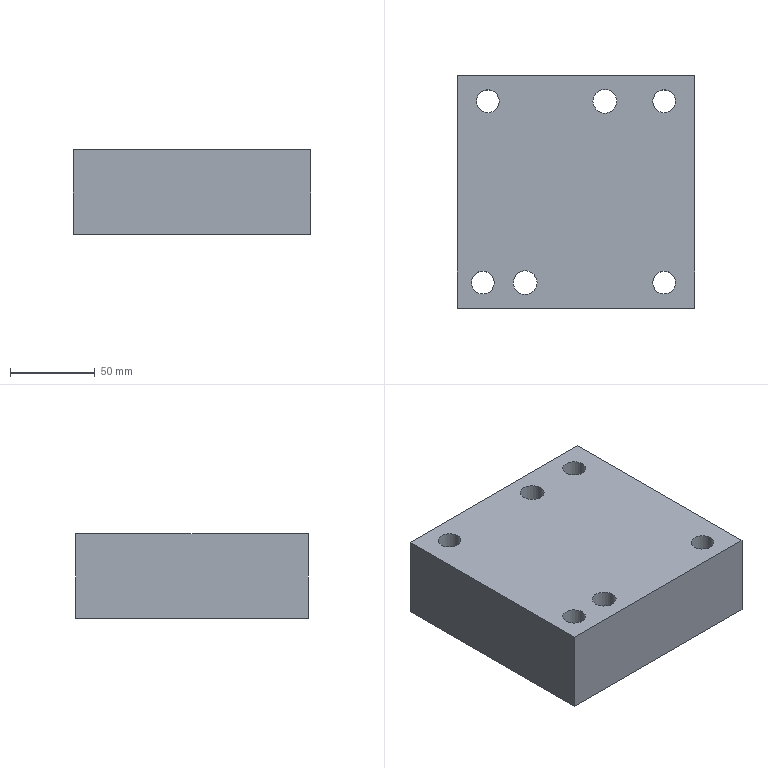Part | STEP file | lll_id3158_x_t | 1 solid | 16 faces | box 140 x 137 x 50 mm | volume 911433 mm3 | cylinder 8 | plane 6 | cone 2 | commonest cylinder face diameters 13.509 x4 8.506 x2 14 x2
STEP:
#1=CARTESIAN_POINT('',(525.125,-377.25,142.5));
#2=VERTEX_POINT('',#1);
#3=CARTESIAN_POINT('',(518.37,-377.25,142.5));
#4=DIRECTION('',(0.,0.,1.));
#5=DIRECTION('',(1.,0.,0.));
#6=AXIS2_PLACEMENT_3D('',#3,#4,#5);
#7=CIRCLE('',#6,6.755);
#8=EDGE_CURVE('',#2,#2,#7,.T.);
#9=ORIENTED_EDGE('',*,*,#8,.F.);
#10=EDGE_LOOP('',(#9));
#11=FACE_BOUND('',#10,.T.);
#12=CARTESIAN_POINT('',(490.371,-270.25,142.5));
#13=VERTEX_POINT('',#12);
#14=CARTESIAN_POINT('',(483.37,-270.25,142.5));
#15=DIRECTION('',(0.,0.,-1.));
#16=DIRECTION('',(1.,0.,0.));
#17=AXIS2_PLACEMENT_3D('',#14,#15,#16);
#18=CIRCLE('',#17,7.);
#19=EDGE_CURVE('',#13,#13,#18,.T.);
#20=ORIENTED_EDGE('',*,*,#19,.T.);
#21=EDGE_LOOP('',(#20));
#22=FACE_BOUND('',#21,.T.);
#23=CARTESIAN_POINT('',(421.125,-270.25,142.5));
#24=VERTEX_POINT('',#23);
#25=CARTESIAN_POINT('',(414.37,-270.25,142.5));
#26=DIRECTION('',(0.,0.,1.));
#27=DIRECTION('',(1.,0.,0.));
#28=AXIS2_PLACEMENT_3D('',#25,#26,#27);
#29=CIRCLE('',#28,6.755);
#30=EDGE_CURVE('',#24,#24,#29,.T.);
#31=ORIENTED_EDGE('',*,*,#30,.F.);
#32=EDGE_LOOP('',(#31));
#33=FACE_BOUND('',#32,.T.);
#34=CARTESIAN_POINT('',(443.371,-377.25,142.5));
#35=VERTEX_POINT('',#34);
#36=CARTESIAN_POINT('',(436.37,-377.25,142.5));
#37=DIRECTION('',(0.,0.,-1.));
#38=DIRECTION('',(1.,0.,0.));
#39=AXIS2_PLACEMENT_3D('',#36,#37,#38);
#40=CIRCLE('',#39,7.);
#41=EDGE_CURVE('',#35,#35,#40,.T.);
#42=ORIENTED_EDGE('',*,*,#41,.T.);
#43=EDGE_LOOP('',(#42));
#44=FACE_BOUND('',#43,.T.);
#45=CARTESIAN_POINT('',(536.37,-255.25,142.5));
#46=VERTEX_POINT('',#45);
#47=CARTESIAN_POINT('',(536.37,-392.25,142.5));
#48=VERTEX_POINT('',#47);
#49=CARTESIAN_POINT('',(536.37,-325.25,142.5));
#50=DIRECTION('',(0.,-1.,0.));
#51=VECTOR('',#50,1.);
#52=LINE('',#49,#51);
#53=EDGE_CURVE('',#46,#48,#52,.T.);
#54=ORIENTED_EDGE('',*,*,#53,.F.);
#55=CARTESIAN_POINT('',(396.37,-255.25,142.5));
#56=VERTEX_POINT('',#55);
#57=CARTESIAN_POINT('',(466.37,-255.25,142.5));
#58=DIRECTION('',(1.,0.,0.));
#59=VECTOR('',#58,1.);
#60=LINE('',#57,#59);
#61=EDGE_CURVE('',#56,#46,#60,.T.);
#62=ORIENTED_EDGE('',*,*,#61,.F.);
#63=CARTESIAN_POINT('',(396.37,-392.25,142.5));
#64=VERTEX_POINT('',#63);
#65=CARTESIAN_POINT('',(396.37,-325.25,142.5));
#66=DIRECTION('',(0.,1.,0.));
#67=VECTOR('',#66,1.);
#68=LINE('',#65,#67);
#69=EDGE_CURVE('',#64,#56,#68,.T.);
#70=ORIENTED_EDGE('',*,*,#69,.F.);
#71=CARTESIAN_POINT('',(466.37,-392.25,142.5));
#72=DIRECTION('',(-1.,0.,0.));
#73=VECTOR('',#72,1.);
#74=LINE('',#71,#73);
#75=EDGE_CURVE('',#48,#64,#74,.T.);
#76=ORIENTED_EDGE('',*,*,#75,.F.);
#77=EDGE_LOOP('',(#54,#62,#70,#76));
#78=FACE_BOUND('',#77,.T.);
#79=CARTESIAN_POINT('',(418.125,-377.25,142.5));
#80=VERTEX_POINT('',#79);
#81=CARTESIAN_POINT('',(411.37,-377.25,142.5));
#82=DIRECTION('',(0.,0.,-1.));
#83=DIRECTION('',(1.,0.,0.));
#84=AXIS2_PLACEMENT_3D('',#81,#82,#83);
#85=CIRCLE('',#84,6.755);
#86=EDGE_CURVE('',#80,#80,#85,.T.);
#87=ORIENTED_EDGE('',*,*,#86,.T.);
#88=EDGE_LOOP('',(#87));
#89=FACE_BOUND('',#88,.T.);
#90=CARTESIAN_POINT('',(525.125,-270.25,142.5));
#91=VERTEX_POINT('',#90);
#92=CARTESIAN_POINT('',(518.37,-270.25,142.5));
#93=DIRECTION('',(0.,0.,-1.));
#94=DIRECTION('',(1.,0.,0.));
#95=AXIS2_PLACEMENT_3D('',#92,#93,#94);
#96=CIRCLE('',#95,6.755);
#97=EDGE_CURVE('',#91,#91,#96,.T.);
#98=ORIENTED_EDGE('',*,*,#97,.T.);
#99=EDGE_LOOP('',(#98));
#100=FACE_BOUND('',#99,.T.);
#101=CARTESIAN_POINT('',(42.419,-273.704,142.5));
#102=DIRECTION('',(0.,0.,1.));
#103=DIRECTION('',(-1.,0.,0.));
#104=AXIS2_PLACEMENT_3D('',#101,#102,#103);
#105=PLANE('',#104);
#106=ADVANCED_FACE('',(#11,#22,#33,#44,#78,#89,#100),#105,.T.);
#107=CARTESIAN_POINT('',(497.123,-320.,92.5));
#108=VERTEX_POINT('',#107);
#109=CARTESIAN_POINT('',(492.87,-320.,92.5));
#110=DIRECTION('',(0.,0.,1.));
#111=DIRECTION('',(1.,0.,0.));
#112=AXIS2_PLACEMENT_3D('',#109,#110,#111);
#113=CIRCLE('',#112,4.253);
#114=EDGE_CURVE('',#108,#108,#113,.T.);
#115=ORIENTED_EDGE('',*,*,#114,.T.);
#116=EDGE_LOOP('',(#115));
#117=FACE_BOUND('',#116,.T.);
#118=CARTESIAN_POINT('',(441.253,-325.5,92.5));
#119=VERTEX_POINT('',#118);
#120=CARTESIAN_POINT('',(437.,-325.5,92.5));
#121=DIRECTION('',(0.,0.,1.));
#122=DIRECTION('',(1.,0.,0.));
#123=AXIS2_PLACEMENT_3D('',#120,#121,#122);
#124=CIRCLE('',#123,4.253);
#125=EDGE_CURVE('',#119,#119,#124,.T.);
#126=ORIENTED_EDGE('',*,*,#125,.T.);
#127=EDGE_LOOP('',(#126));
#128=FACE_BOUND('',#127,.T.);
#129=CARTESIAN_POINT('',(511.616,-377.25,92.5));
#130=VERTEX_POINT('',#129);
#131=CARTESIAN_POINT('',(518.37,-377.25,92.5));
#132=DIRECTION('',(0.,0.,-1.));
#133=DIRECTION('',(-1.,0.,0.));
#134=AXIS2_PLACEMENT_3D('',#131,#132,#133);
#135=CIRCLE('',#134,6.755);
#136=EDGE_CURVE('',#130,#130,#135,.T.);
#137=ORIENTED_EDGE('',*,*,#136,.F.);
#138=EDGE_LOOP('',(#137));
#139=FACE_BOUND('',#138,.T.);
#140=CARTESIAN_POINT('',(511.616,-270.25,92.5));
#141=VERTEX_POINT('',#140);
#142=CARTESIAN_POINT('',(518.37,-270.25,92.5));
#143=DIRECTION('',(0.,0.,-1.));
#144=DIRECTION('',(-1.,0.,0.));
#145=AXIS2_PLACEMENT_3D('',#142,#143,#144);
#146=CIRCLE('',#145,6.755);
#147=EDGE_CURVE('',#141,#141,#146,.T.);
#148=ORIENTED_EDGE('',*,*,#147,.F.);
#149=EDGE_LOOP('',(#148));
#150=FACE_BOUND('',#149,.T.);
#151=CARTESIAN_POINT('',(429.37,-377.25,92.5));
#152=VERTEX_POINT('',#151);
#153=CARTESIAN_POINT('',(436.37,-377.25,92.5));
#154=DIRECTION('',(0.,0.,1.));
#155=DIRECTION('',(-1.,0.,0.));
#156=AXIS2_PLACEMENT_3D('',#153,#154,#155);
#157=CIRCLE('',#156,7.);
#158=EDGE_CURVE('',#152,#152,#157,.T.);
#159=ORIENTED_EDGE('',*,*,#158,.T.);
#160=EDGE_LOOP('',(#159));
#161=FACE_BOUND('',#160,.T.);
#162=CARTESIAN_POINT('',(536.37,-255.25,92.5));
#163=VERTEX_POINT('',#162);
#164=CARTESIAN_POINT('',(396.37,-255.25,92.5));
#165=VERTEX_POINT('',#164);
#166=CARTESIAN_POINT('',(466.37,-255.25,92.5));
#167=DIRECTION('',(-1.,0.,0.));
#168=VECTOR('',#167,1.);
#169=LINE('',#166,#168);
#170=EDGE_CURVE('',#163,#165,#169,.T.);
#171=ORIENTED_EDGE('',*,*,#170,.F.);
#172=CARTESIAN_POINT('',(536.37,-392.25,92.5));
#173=VERTEX_POINT('',#172);
#174=CARTESIAN_POINT('',(536.37,-325.25,92.5));
#175=DIRECTION('',(0.,1.,0.));
#176=VECTOR('',#175,1.);
#177=LINE('',#174,#176);
#178=EDGE_CURVE('',#173,#163,#177,.T.);
#179=ORIENTED_EDGE('',*,*,#178,.F.);
#180=CARTESIAN_POINT('',(396.37,-392.25,92.5));
#181=VERTEX_POINT('',#180);
#182=CARTESIAN_POINT('',(466.37,-392.25,92.5));
#183=DIRECTION('',(1.,0.,0.));
#184=VECTOR('',#183,1.);
#185=LINE('',#182,#184);
#186=EDGE_CURVE('',#181,#173,#185,.T.);
#187=ORIENTED_EDGE('',*,*,#186,.F.);
#188=CARTESIAN_POINT('',(396.37,-325.25,92.5));
#189=DIRECTION('',(0.,-1.,0.));
#190=VECTOR('',#189,1.);
#191=LINE('',#188,#190);
#192=EDGE_CURVE('',#165,#181,#191,.T.);
#193=ORIENTED_EDGE('',*,*,#192,.F.);
#194=EDGE_LOOP('',(#171,#179,#187,#193));
#195=FACE_BOUND('',#194,.T.);
#196=CARTESIAN_POINT('',(404.616,-377.25,92.5));
#197=VERTEX_POINT('',#196);
#198=CARTESIAN_POINT('',(411.37,-377.25,92.5));
#199=DIRECTION('',(0.,0.,-1.));
#200=DIRECTION('',(-1.,0.,0.));
#201=AXIS2_PLACEMENT_3D('',#198,#199,#200);
#202=CIRCLE('',#201,6.755);
#203=EDGE_CURVE('',#197,#197,#202,.T.);
#204=ORIENTED_EDGE('',*,*,#203,.F.);
#205=EDGE_LOOP('',(#204));
#206=FACE_BOUND('',#205,.T.);
#207=CARTESIAN_POINT('',(407.616,-270.25,92.5));
#208=VERTEX_POINT('',#207);
#209=CARTESIAN_POINT('',(414.37,-270.25,92.5));
#210=DIRECTION('',(0.,0.,-1.));
#211=DIRECTION('',(-1.,0.,0.));
#212=AXIS2_PLACEMENT_3D('',#209,#210,#211);
#213=CIRCLE('',#212,6.755);
#214=EDGE_CURVE('',#208,#208,#213,.T.);
#215=ORIENTED_EDGE('',*,*,#214,.F.);
#216=EDGE_LOOP('',(#215));
#217=FACE_BOUND('',#216,.T.);
#218=CARTESIAN_POINT('',(490.371,-270.25,92.5));
#219=VERTEX_POINT('',#218);
#220=CARTESIAN_POINT('',(483.37,-270.25,92.5));
#221=DIRECTION('',(0.,0.,1.));
#222=DIRECTION('',(1.,0.,0.));
#223=AXIS2_PLACEMENT_3D('',#220,#221,#222);
#224=CIRCLE('',#223,7.);
#225=EDGE_CURVE('',#219,#219,#224,.T.);
#226=ORIENTED_EDGE('',*,*,#225,.T.);
#227=EDGE_LOOP('',(#226));
#228=FACE_BOUND('',#227,.T.);
#229=CARTESIAN_POINT('',(466.37,-325.25,92.5));
#230=DIRECTION('',(0.,0.,-1.));
#231=DIRECTION('',(0.,-1.,0.));
#232=AXIS2_PLACEMENT_3D('',#229,#230,#231);
#233=PLANE('',#232);
#234=ADVANCED_FACE('',(#117,#128,#139,#150,#161,#195,#206,#217,#228),#233,.T.);
#235=CARTESIAN_POINT('',(536.37,-255.25,92.5));
#236=DIRECTION('',(0.,0.,1.));
#237=VECTOR('',#236,1.);
#238=LINE('',#235,#237);
#239=EDGE_CURVE('',#163,#46,#238,.T.);
#240=ORIENTED_EDGE('',*,*,#239,.T.);
#241=ORIENTED_EDGE('',*,*,#53,.T.);
#242=CARTESIAN_POINT('',(536.37,-392.25,92.5));
#243=DIRECTION('',(0.,0.,1.));
#244=VECTOR('',#243,1.);
#245=LINE('',#242,#244);
#246=EDGE_CURVE('',#173,#48,#245,.T.);
#247=ORIENTED_EDGE('',*,*,#246,.F.);
#248=ORIENTED_EDGE('',*,*,#178,.T.);
#249=EDGE_LOOP('',(#240,#241,#247,#248));
#250=FACE_OUTER_BOUND('',#249,.T.);
#251=CARTESIAN_POINT('',(536.37,-325.25,92.5));
#252=DIRECTION('',(1.,0.,0.));
#253=DIRECTION('',(0.,0.,-1.));
#254=AXIS2_PLACEMENT_3D('',#251,#252,#253);
#255=PLANE('',#254);
#256=ADVANCED_FACE('',(#250),#255,.T.);
#257=ORIENTED_EDGE('',*,*,#246,.T.);
#258=ORIENTED_EDGE('',*,*,#75,.T.);
#259=CARTESIAN_POINT('',(396.37,-392.25,92.5));
#260=DIRECTION('',(0.,0.,1.));
#261=VECTOR('',#260,1.);
#262=LINE('',#259,#261);
#263=EDGE_CURVE('',#181,#64,#262,.T.);
#264=ORIENTED_EDGE('',*,*,#263,.F.);
#265=ORIENTED_EDGE('',*,*,#186,.T.);
#266=EDGE_LOOP('',(#257,#258,#264,#265));
#267=FACE_OUTER_BOUND('',#266,.T.);
#268=CARTESIAN_POINT('',(466.37,-392.25,92.5));
#269=DIRECTION('',(0.,-1.,0.));
#270=DIRECTION('',(0.,0.,1.));
#271=AXIS2_PLACEMENT_3D('',#268,#269,#270);
#272=PLANE('',#271);
#273=ADVANCED_FACE('',(#267),#272,.T.);
#274=ORIENTED_EDGE('',*,*,#263,.T.);
#275=ORIENTED_EDGE('',*,*,#69,.T.);
#276=CARTESIAN_POINT('',(396.37,-255.25,92.5));
#277=DIRECTION('',(0.,0.,1.));
#278=VECTOR('',#277,1.);
#279=LINE('',#276,#278);
#280=EDGE_CURVE('',#165,#56,#279,.T.);
#281=ORIENTED_EDGE('',*,*,#280,.F.);
#282=ORIENTED_EDGE('',*,*,#192,.T.);
#283=EDGE_LOOP('',(#274,#275,#281,#282));
#284=FACE_OUTER_BOUND('',#283,.T.);
#285=CARTESIAN_POINT('',(396.37,-325.25,92.5));
#286=DIRECTION('',(-1.,0.,0.));
#287=DIRECTION('',(0.,0.,1.));
#288=AXIS2_PLACEMENT_3D('',#285,#286,#287);
#289=PLANE('',#288);
#290=ADVANCED_FACE('',(#284),#289,.T.);
#291=ORIENTED_EDGE('',*,*,#170,.T.);
#292=ORIENTED_EDGE('',*,*,#280,.T.);
#293=ORIENTED_EDGE('',*,*,#61,.T.);
#294=ORIENTED_EDGE('',*,*,#239,.F.);
#295=EDGE_LOOP('',(#291,#292,#293,#294));
#296=FACE_OUTER_BOUND('',#295,.T.);
#297=CARTESIAN_POINT('',(466.37,-255.25,92.5));
#298=DIRECTION('',(0.,1.,0.));
#299=DIRECTION('',(0.,0.,-1.));
#300=AXIS2_PLACEMENT_3D('',#297,#298,#299);
#301=PLANE('',#300);
#302=ADVANCED_FACE('',(#296),#301,.T.);
#303=ORIENTED_EDGE('',*,*,#41,.F.);
#304=EDGE_LOOP('',(#303));
#305=FACE_BOUND('',#304,.T.);
#306=ORIENTED_EDGE('',*,*,#158,.F.);
#307=EDGE_LOOP('',(#306));
#308=FACE_BOUND('',#307,.T.);
#309=CARTESIAN_POINT('',(436.37,-377.25,92.5));
#310=DIRECTION('',(0.,0.,1.));
#311=DIRECTION('',(-1.,0.,0.));
#312=AXIS2_PLACEMENT_3D('',#309,#310,#311);
#313=CYLINDRICAL_SURFACE('',#312,7.);
#314=ADVANCED_FACE('',(#305,#308),#313,.F.);
#315=ORIENTED_EDGE('',*,*,#203,.T.);
#316=EDGE_LOOP('',(#315));
#317=FACE_BOUND('',#316,.T.);
#318=ORIENTED_EDGE('',*,*,#86,.F.);
#319=EDGE_LOOP('',(#318));
#320=FACE_BOUND('',#319,.T.);
#321=CARTESIAN_POINT('',(411.37,-377.25,57.5));
#322=DIRECTION('',(0.,0.,1.));
#323=DIRECTION('',(-1.,0.,0.));
#324=AXIS2_PLACEMENT_3D('',#321,#322,#323);
#325=CYLINDRICAL_SURFACE('',#324,6.755);
#326=ADVANCED_FACE('',(#317,#320),#325,.F.);
#327=ORIENTED_EDGE('',*,*,#214,.T.);
#328=EDGE_LOOP('',(#327));
#329=FACE_BOUND('',#328,.T.);
#330=ORIENTED_EDGE('',*,*,#30,.T.);
#331=EDGE_LOOP('',(#330));
#332=FACE_BOUND('',#331,.T.);
#333=CARTESIAN_POINT('',(414.37,-270.25,57.5));
#334=DIRECTION('',(0.,0.,1.));
#335=DIRECTION('',(-1.,0.,0.));
#336=AXIS2_PLACEMENT_3D('',#333,#334,#335);
#337=CYLINDRICAL_SURFACE('',#336,6.755);
#338=ADVANCED_FACE('',(#329,#332),#337,.F.);
#339=ORIENTED_EDGE('',*,*,#19,.F.);
#340=EDGE_LOOP('',(#339));
#341=FACE_BOUND('',#340,.T.);
#342=ORIENTED_EDGE('',*,*,#225,.F.);
#343=EDGE_LOOP('',(#342));
#344=FACE_BOUND('',#343,.T.);
#345=CARTESIAN_POINT('',(483.37,-270.25,92.5));
#346=DIRECTION('',(0.,0.,1.));
#347=DIRECTION('',(1.,0.,0.));
#348=AXIS2_PLACEMENT_3D('',#345,#346,#347);
#349=CYLINDRICAL_SURFACE('',#348,7.);
#350=ADVANCED_FACE('',(#341,#344),#349,.F.);
#351=ORIENTED_EDGE('',*,*,#147,.T.);
#352=EDGE_LOOP('',(#351));
#353=FACE_BOUND('',#352,.T.);
#354=ORIENTED_EDGE('',*,*,#97,.F.);
#355=EDGE_LOOP('',(#354));
#356=FACE_BOUND('',#355,.T.);
#357=CARTESIAN_POINT('',(518.37,-270.25,57.5));
#358=DIRECTION('',(0.,0.,1.));
#359=DIRECTION('',(1.,0.,0.));
#360=AXIS2_PLACEMENT_3D('',#357,#358,#359);
#361=CYLINDRICAL_SURFACE('',#360,6.755);
#362=ADVANCED_FACE('',(#353,#356),#361,.F.);
#363=ORIENTED_EDGE('',*,*,#136,.T.);
#364=EDGE_LOOP('',(#363));
#365=FACE_BOUND('',#364,.T.);
#366=ORIENTED_EDGE('',*,*,#8,.T.);
#367=EDGE_LOOP('',(#366));
#368=FACE_BOUND('',#367,.T.);
#369=CARTESIAN_POINT('',(518.37,-377.25,57.5));
#370=DIRECTION('',(0.,0.,1.));
#371=DIRECTION('',(1.,0.,0.));
#372=AXIS2_PLACEMENT_3D('',#369,#370,#371);
#373=CYLINDRICAL_SURFACE('',#372,6.755);
#374=ADVANCED_FACE('',(#365,#368),#373,.F.);
#375=CARTESIAN_POINT('',(441.253,-325.5,122.5));
#376=VERTEX_POINT('',#375);
#377=CARTESIAN_POINT('',(437.,-325.5,122.5));
#378=DIRECTION('',(0.,0.,-1.));
#379=DIRECTION('',(1.,0.,0.));
#380=AXIS2_PLACEMENT_3D('',#377,#378,#379);
#381=CIRCLE('',#380,4.253);
#382=EDGE_CURVE('',#376,#376,#381,.T.);
#383=ORIENTED_EDGE('',*,*,#382,.T.);
#384=EDGE_LOOP('',(#383));
#385=FACE_BOUND('',#384,.T.);
#386=CARTESIAN_POINT('',(437.,-325.5,125.055));
#387=VERTEX_POINT('',#386);
#388=VERTEX_LOOP('',#387);
#389=FACE_BOUND('',#388,.T.);
#390=CARTESIAN_POINT('',(437.,-325.5,122.5));
#391=DIRECTION('',(0.,0.,-1.));
#392=DIRECTION('',(1.,0.,0.));
#393=AXIS2_PLACEMENT_3D('',#390,#391,#392);
#394=CONICAL_SURFACE('',#393,4.253,59.);
#395=ADVANCED_FACE('',(#385,#389),#394,.F.);
#396=ORIENTED_EDGE('',*,*,#382,.F.);
#397=EDGE_LOOP('',(#396));
#398=FACE_BOUND('',#397,.T.);
#399=ORIENTED_EDGE('',*,*,#125,.F.);
#400=EDGE_LOOP('',(#399));
#401=FACE_BOUND('',#400,.T.);
#402=CARTESIAN_POINT('',(437.,-325.5,92.5));
#403=DIRECTION('',(0.,0.,1.));
#404=DIRECTION('',(-1.,0.,0.));
#405=AXIS2_PLACEMENT_3D('',#402,#403,#404);
#406=CYLINDRICAL_SURFACE('',#405,4.253);
#407=ADVANCED_FACE('',(#398,#401),#406,.F.);
#408=CARTESIAN_POINT('',(497.123,-320.,122.5));
#409=VERTEX_POINT('',#408);
#410=CARTESIAN_POINT('',(492.87,-320.,122.5));
#411=DIRECTION('',(0.,0.,-1.));
#412=DIRECTION('',(1.,0.,0.));
#413=AXIS2_PLACEMENT_3D('',#410,#411,#412);
#414=CIRCLE('',#413,4.253);
#415=EDGE_CURVE('',#409,#409,#414,.T.);
#416=ORIENTED_EDGE('',*,*,#415,.T.);
#417=EDGE_LOOP('',(#416));
#418=FACE_BOUND('',#417,.T.);
#419=CARTESIAN_POINT('',(492.87,-320.,125.055));
#420=VERTEX_POINT('',#419);
#421=VERTEX_LOOP('',#420);
#422=FACE_BOUND('',#421,.T.);
#423=CARTESIAN_POINT('',(492.87,-320.,122.5));
#424=DIRECTION('',(0.,0.,-1.));
#425=DIRECTION('',(1.,0.,0.));
#426=AXIS2_PLACEMENT_3D('',#423,#424,#425);
#427=CONICAL_SURFACE('',#426,4.253,59.);
#428=ADVANCED_FACE('',(#418,#422),#427,.F.);
#429=ORIENTED_EDGE('',*,*,#415,.F.);
#430=EDGE_LOOP('',(#429));
#431=FACE_BOUND('',#430,.T.);
#432=ORIENTED_EDGE('',*,*,#114,.F.);
#433=EDGE_LOOP('',(#432));
#434=FACE_BOUND('',#433,.T.);
#435=CARTESIAN_POINT('',(492.87,-320.,92.5));
#436=DIRECTION('',(0.,0.,1.));
#437=DIRECTION('',(-1.,0.,0.));
#438=AXIS2_PLACEMENT_3D('',#435,#436,#437);
#439=CYLINDRICAL_SURFACE('',#438,4.253);
#440=ADVANCED_FACE('',(#431,#434),#439,.F.);
#441=CLOSED_SHELL('',(#106,#234,#256,#273,#290,#302,#314,#326,#338,#350,#362,#374,#395,#407,#428,#440));
#442=MANIFOLD_SOLID_BREP('',#441);
#443=(LENGTH_UNIT()NAMED_UNIT(*)SI_UNIT(.MILLI.,.METRE.));
#444=UNCERTAINTY_MEASURE_WITH_UNIT(LENGTH_MEASURE(0.00002),#443,'','');
#445=(NAMED_UNIT(*)PLANE_ANGLE_UNIT()SI_UNIT($,.RADIAN.));
#446=PLANE_ANGLE_MEASURE_WITH_UNIT(PLANE_ANGLE_MEASURE(0.01745),#445);
#447=DIMENSIONAL_EXPONENTS(0.,0.,0.,0.,0.,0.,0.);
#448=(CONVERSION_BASED_UNIT('DEGREE',#446)NAMED_UNIT(#447)PLANE_ANGLE_UNIT());
#449=(NAMED_UNIT(*)SI_UNIT($,.STERADIAN.)SOLID_ANGLE_UNIT());
#450=(GEOMETRIC_REPRESENTATION_CONTEXT(3)GLOBAL_UNCERTAINTY_ASSIGNED_CONTEXT((#444))GLOBAL_UNIT_ASSIGNED_CONTEXT((#443,#448,#449))REPRESENTATION_CONTEXT('',''));
#451=ADVANCED_BREP_SHAPE_REPRESENTATION('',(#442),#450);